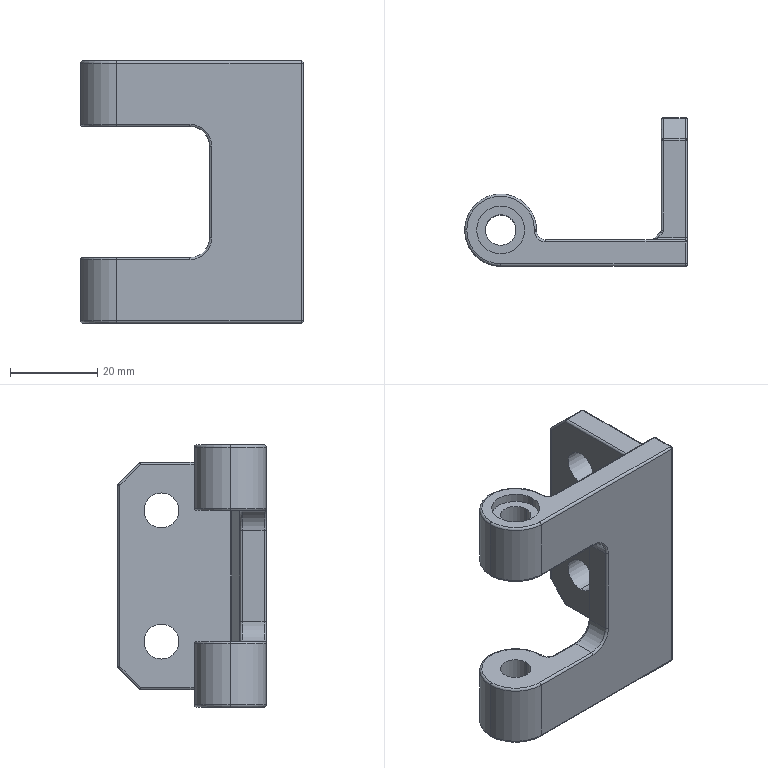Part | STEP file | Hinge base | 1 solid | 117 faces | box 51 x 34 x 60 mm | volume 23679 mm3 | cylinder 59 | torus 27 | plane 17 | sphere 12 | spline 2 | commonest cylinder face diameters 1 x35 16.5 x6 4 x4 7 x4 8 x4 11 x4